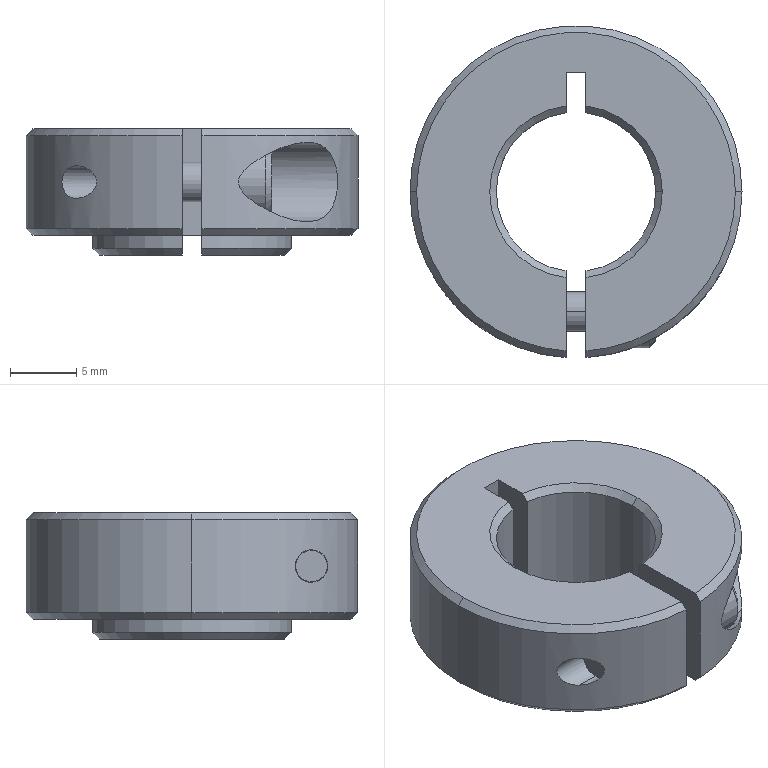Part | NX | features BREP 1 | 1 solid | 58 faces | box 25 x 24.977 x 9.5 mm | volume 2867 mm3 | plane 20 | cone 19 | cylinder 19 | commonest cylinder face diameters 12 x3 15 x3 25 x3 2.459 x2 3 x2 3.5 x2